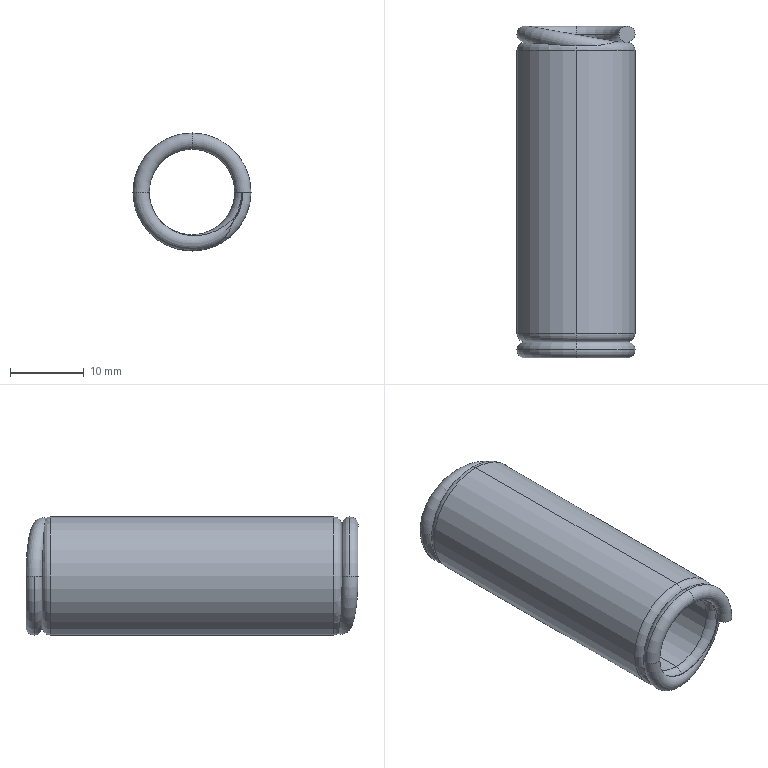Part | SolidWorks | features Revolution 5, RevCut 1 | 1 solid | 30 faces | box 16 x 45 x 16 mm | volume 4068 mm3 | torus 22 | cylinder 4 | plane 4 | commonest cylinder face diameters 11.6 x2 16 x2
STEP:
#1=CARTESIAN_POINT('',(0.,-21.4,8.));
#2=VERTEX_POINT('',#1);
#3=CARTESIAN_POINT('',(0.,-21.4,5.8));
#4=VERTEX_POINT('',#3);
#5=CARTESIAN_POINT('',(0.,-21.4,6.9));
#6=DIRECTION('',(1.,0.,0.));
#7=DIRECTION('',(0.,0.,-1.));
#8=AXIS2_PLACEMENT_3D('',#5,#6,#7);
#9=CIRCLE('',#8,1.1);
#10=EDGE_CURVE('',#2,#4,#9,.T.);
#11=ORIENTED_EDGE('',*,*,#10,.F.);
#12=CARTESIAN_POINT('',(-8.,-21.4,0.));
#13=VERTEX_POINT('',#12);
#14=CARTESIAN_POINT('',(0.,-21.4,0.));
#15=DIRECTION('',(0.,-1.,0.));
#16=DIRECTION('',(0.,0.,-1.));
#17=AXIS2_PLACEMENT_3D('',#14,#15,#16);
#18=CIRCLE('',#17,8.);
#19=EDGE_CURVE('',#2,#13,#18,.T.);
#20=ORIENTED_EDGE('',*,*,#19,.T.);
#21=CARTESIAN_POINT('',(-5.8,-21.4,0.));
#22=VERTEX_POINT('',#21);
#23=CARTESIAN_POINT('',(-6.9,-21.4,0.));
#24=DIRECTION('',(0.,0.,1.));
#25=DIRECTION('',(1.,0.,0.));
#26=AXIS2_PLACEMENT_3D('',#23,#24,#25);
#27=CIRCLE('',#26,1.1);
#28=EDGE_CURVE('',#13,#22,#27,.T.);
#29=ORIENTED_EDGE('',*,*,#28,.T.);
#30=CARTESIAN_POINT('',(0.,-21.4,0.));
#31=DIRECTION('',(0.,-1.,0.));
#32=DIRECTION('',(0.,0.,-1.));
#33=AXIS2_PLACEMENT_3D('',#30,#31,#32);
#34=CIRCLE('',#33,5.8);
#35=EDGE_CURVE('',#4,#22,#34,.T.);
#36=ORIENTED_EDGE('',*,*,#35,.F.);
#37=EDGE_LOOP('',(#11,#20,#29,#36));
#38=FACE_OUTER_BOUND('',#37,.T.);
#39=CARTESIAN_POINT('',(0.,-21.4,0.));
#40=DIRECTION('',(0.,-1.,0.));
#41=DIRECTION('',(0.,0.,-1.));
#42=AXIS2_PLACEMENT_3D('',#39,#40,#41);
#43=TOROIDAL_SURFACE('',#42,6.9,1.1);
#44=ADVANCED_FACE('',(#38),#43,.T.);
#45=CARTESIAN_POINT('',(0.,-20.3,6.9));
#46=VERTEX_POINT('',#45);
#47=CARTESIAN_POINT('',(0.,-21.4,6.9));
#48=DIRECTION('',(1.,0.,0.));
#49=DIRECTION('',(0.,0.,-1.));
#50=AXIS2_PLACEMENT_3D('',#47,#48,#49);
#51=CIRCLE('',#50,1.1);
#52=EDGE_CURVE('',#4,#46,#51,.T.);
#53=ORIENTED_EDGE('',*,*,#52,.F.);
#54=ORIENTED_EDGE('',*,*,#35,.T.);
#55=CARTESIAN_POINT('',(0.,-20.877,-5.932));
#56=VERTEX_POINT('',#55);
#57=CARTESIAN_POINT('',(0.,-20.877,-5.932));
#58=CARTESIAN_POINT('',(-0.3787,-20.912,-5.913));
#59=CARTESIAN_POINT('',(-0.7536,-20.947,-5.861));
#60=CARTESIAN_POINT('',(-1.31,-20.997,-5.731));
#61=CARTESIAN_POINT('',(-1.496,-21.014,-5.679));
#62=CARTESIAN_POINT('',(-1.858,-21.047,-5.559));
#63=CARTESIAN_POINT('',(-2.035,-21.063,-5.491));
#64=CARTESIAN_POINT('',(-2.556,-21.111,-5.263));
#65=CARTESIAN_POINT('',(-2.888,-21.141,-5.08));
#66=CARTESIAN_POINT('',(-3.522,-21.198,-4.647));
#67=CARTESIAN_POINT('',(-3.815,-21.224,-4.403));
#68=CARTESIAN_POINT('',(-4.217,-21.26,-4.));
#69=CARTESIAN_POINT('',(-4.344,-21.271,-3.859));
#70=CARTESIAN_POINT('',(-4.587,-21.293,-3.563));
#71=CARTESIAN_POINT('',(-4.702,-21.303,-3.408));
#72=CARTESIAN_POINT('',(-5.021,-21.331,-2.932));
#73=CARTESIAN_POINT('',(-5.201,-21.347,-2.598));
#74=CARTESIAN_POINT('',(-5.495,-21.373,-1.895));
#75=CARTESIAN_POINT('',(-5.609,-21.383,-1.525));
#76=CARTESIAN_POINT('',(-5.762,-21.397,-0.77));
#77=CARTESIAN_POINT('',(-5.8,-21.4,-0.3815));
#78=CARTESIAN_POINT('',(-5.8,-21.4,0.));
#79=B_SPLINE_CURVE_WITH_KNOTS('',3,(#57,#58,#59,#60,#61,#62,#63,#64,#65,#66,#67,#68,#69,#70,#71,#72,#73,#74,#75,#76,#77,#78),.UNSPECIFIED.,.F.,.F.,(4,2,2,2,2,2,2,2,2,2,4),(0.01087,0.01202,0.01259,0.01316,0.01431,0.01545,0.01602,0.01659,0.01774,0.01888,0.02003),.UNSPECIFIED.);
#80=EDGE_CURVE('',#56,#22,#79,.T.);
#81=ORIENTED_EDGE('',*,*,#80,.F.);
#82=CARTESIAN_POINT('',(0.,-20.3,-6.9));
#83=VERTEX_POINT('',#82);
#84=CARTESIAN_POINT('',(0.,-21.4,-6.9));
#85=DIRECTION('',(-1.,0.,0.));
#86=DIRECTION('',(0.,0.,1.));
#87=AXIS2_PLACEMENT_3D('',#84,#85,#86);
#88=CIRCLE('',#87,1.1);
#89=EDGE_CURVE('',#56,#83,#88,.T.);
#90=ORIENTED_EDGE('',*,*,#89,.T.);
#91=CARTESIAN_POINT('',(0.,-20.3,0.));
#92=DIRECTION('',(0.,1.,0.));
#93=DIRECTION('',(0.,0.,1.));
#94=AXIS2_PLACEMENT_3D('',#91,#92,#93);
#95=CIRCLE('',#94,6.9);
#96=EDGE_CURVE('',#83,#46,#95,.T.);
#97=ORIENTED_EDGE('',*,*,#96,.T.);
#98=EDGE_LOOP('',(#53,#54,#81,#90,#97));
#99=FACE_OUTER_BOUND('',#98,.T.);
#100=CARTESIAN_POINT('',(0.,-21.4,0.));
#101=DIRECTION('',(0.,-1.,0.));
#102=DIRECTION('',(0.,0.,-1.));
#103=AXIS2_PLACEMENT_3D('',#100,#101,#102);
#104=TOROIDAL_SURFACE('',#103,6.9,1.1);
#105=ADVANCED_FACE('',(#99),#104,.T.);
#106=CARTESIAN_POINT('',(0.,21.4,-8.));
#107=VERTEX_POINT('',#106);
#108=CARTESIAN_POINT('',(0.,21.4,-5.8));
#109=VERTEX_POINT('',#108);
#110=CARTESIAN_POINT('',(0.,21.4,-6.9));
#111=DIRECTION('',(1.,0.,0.));
#112=DIRECTION('',(0.,0.,-1.));
#113=AXIS2_PLACEMENT_3D('',#110,#111,#112);
#114=CIRCLE('',#113,1.1);
#115=EDGE_CURVE('',#107,#109,#114,.T.);
#116=ORIENTED_EDGE('',*,*,#115,.F.);
#117=CARTESIAN_POINT('',(-8.,21.4,0.));
#118=VERTEX_POINT('',#117);
#119=CARTESIAN_POINT('',(0.,21.4,0.));
#120=DIRECTION('',(0.,1.,0.));
#121=DIRECTION('',(0.,0.,1.));
#122=AXIS2_PLACEMENT_3D('',#119,#120,#121);
#123=CIRCLE('',#122,8.);
#124=EDGE_CURVE('',#107,#118,#123,.T.);
#125=ORIENTED_EDGE('',*,*,#124,.T.);
#126=CARTESIAN_POINT('',(-5.8,21.4,0.));
#127=VERTEX_POINT('',#126);
#128=CARTESIAN_POINT('',(-6.9,21.4,0.));
#129=DIRECTION('',(0.,0.,1.));
#130=DIRECTION('',(1.,0.,0.));
#131=AXIS2_PLACEMENT_3D('',#128,#129,#130);
#132=CIRCLE('',#131,1.1);
#133=EDGE_CURVE('',#127,#118,#132,.T.);
#134=ORIENTED_EDGE('',*,*,#133,.F.);
#135=CARTESIAN_POINT('',(0.,21.4,0.));
#136=DIRECTION('',(0.,1.,0.));
#137=DIRECTION('',(0.,0.,1.));
#138=AXIS2_PLACEMENT_3D('',#135,#136,#137);
#139=CIRCLE('',#138,5.8);
#140=EDGE_CURVE('',#109,#127,#139,.T.);
#141=ORIENTED_EDGE('',*,*,#140,.F.);
#142=EDGE_LOOP('',(#116,#125,#134,#141));
#143=FACE_OUTER_BOUND('',#142,.T.);
#144=CARTESIAN_POINT('',(0.,21.4,0.));
#145=DIRECTION('',(0.,1.,0.));
#146=DIRECTION('',(0.,0.,1.));
#147=AXIS2_PLACEMENT_3D('',#144,#145,#146);
#148=TOROIDAL_SURFACE('',#147,6.9,1.1);
#149=ADVANCED_FACE('',(#143),#148,.T.);
#150=CARTESIAN_POINT('',(0.,20.3,-6.9));
#151=VERTEX_POINT('',#150);
#152=CARTESIAN_POINT('',(0.,21.4,-6.9));
#153=DIRECTION('',(1.,0.,0.));
#154=DIRECTION('',(0.,0.,-1.));
#155=AXIS2_PLACEMENT_3D('',#152,#153,#154);
#156=CIRCLE('',#155,1.1);
#157=EDGE_CURVE('',#109,#151,#156,.T.);
#158=ORIENTED_EDGE('',*,*,#157,.F.);
#159=ORIENTED_EDGE('',*,*,#140,.T.);
#160=CARTESIAN_POINT('',(0.,20.877,5.932));
#161=VERTEX_POINT('',#160);
#162=CARTESIAN_POINT('',(-5.8,21.4,0.));
#163=CARTESIAN_POINT('',(-5.8,21.4,0.3854));
#164=CARTESIAN_POINT('',(-5.761,21.397,0.7711));
#165=CARTESIAN_POINT('',(-5.609,21.383,1.526));
#166=CARTESIAN_POINT('',(-5.495,21.373,1.896));
#167=CARTESIAN_POINT('',(-5.201,21.347,2.598));
#168=CARTESIAN_POINT('',(-5.021,21.331,2.933));
#169=CARTESIAN_POINT('',(-4.702,21.303,3.409));
#170=CARTESIAN_POINT('',(-4.586,21.293,3.564));
#171=CARTESIAN_POINT('',(-4.344,21.271,3.859));
#172=CARTESIAN_POINT('',(-4.216,21.26,4.));
#173=CARTESIAN_POINT('',(-3.815,21.224,4.404));
#174=CARTESIAN_POINT('',(-3.522,21.198,4.647));
#175=CARTESIAN_POINT('',(-2.888,21.141,5.08));
#176=CARTESIAN_POINT('',(-2.555,21.111,5.263));
#177=CARTESIAN_POINT('',(-2.035,21.063,5.491));
#178=CARTESIAN_POINT('',(-1.857,21.047,5.559));
#179=CARTESIAN_POINT('',(-1.496,21.014,5.679));
#180=CARTESIAN_POINT('',(-1.31,20.997,5.731));
#181=CARTESIAN_POINT('',(-0.7535,20.947,5.861));
#182=CARTESIAN_POINT('',(-0.3786,20.912,5.913));
#183=CARTESIAN_POINT('',(0.,20.877,5.932));
#184=B_SPLINE_CURVE_WITH_KNOTS('',3,(#162,#163,#164,#165,#166,#167,#168,#169,#170,#171,#172,#173,#174,#175,#176,#177,#178,#179,#180,#181,#182,#183),.UNSPECIFIED.,.F.,.F.,(4,2,2,2,2,2,2,2,2,2,4),(-0.0001166,0.001039,0.002196,0.003352,0.00393,0.004508,0.005664,0.00682,0.007398,0.007976,0.009132),.UNSPECIFIED.);
#185=EDGE_CURVE('',#127,#161,#184,.T.);
#186=ORIENTED_EDGE('',*,*,#185,.T.);
#187=CARTESIAN_POINT('',(0.,20.3,6.9));
#188=VERTEX_POINT('',#187);
#189=CARTESIAN_POINT('',(0.,21.4,6.9));
#190=DIRECTION('',(-1.,0.,0.));
#191=DIRECTION('',(0.,0.,1.));
#192=AXIS2_PLACEMENT_3D('',#189,#190,#191);
#193=CIRCLE('',#192,1.1);
#194=EDGE_CURVE('',#161,#188,#193,.T.);
#195=ORIENTED_EDGE('',*,*,#194,.T.);
#196=CARTESIAN_POINT('',(0.,20.3,0.));
#197=DIRECTION('',(0.,1.,0.));
#198=DIRECTION('',(0.,0.,1.));
#199=AXIS2_PLACEMENT_3D('',#196,#197,#198);
#200=CIRCLE('',#199,6.9);
#201=EDGE_CURVE('',#151,#188,#200,.T.);
#202=ORIENTED_EDGE('',*,*,#201,.F.);
#203=EDGE_LOOP('',(#158,#159,#186,#195,#202));
#204=FACE_OUTER_BOUND('',#203,.T.);
#205=CARTESIAN_POINT('',(0.,21.4,0.));
#206=DIRECTION('',(0.,1.,0.));
#207=DIRECTION('',(0.,0.,1.));
#208=AXIS2_PLACEMENT_3D('',#205,#206,#207);
#209=TOROIDAL_SURFACE('',#208,6.9,1.1);
#210=ADVANCED_FACE('',(#204),#209,.T.);
#211=CARTESIAN_POINT('',(5.8,21.4,0.));
#212=VERTEX_POINT('',#211);
#213=CARTESIAN_POINT('',(8.,21.4,0.));
#214=VERTEX_POINT('',#213);
#215=CARTESIAN_POINT('',(6.9,21.4,0.));
#216=DIRECTION('',(0.,0.,-1.));
#217=DIRECTION('',(-1.,0.,0.));
#218=AXIS2_PLACEMENT_3D('',#215,#216,#217);
#219=CIRCLE('',#218,1.1);
#220=EDGE_CURVE('',#212,#214,#219,.T.);
#221=ORIENTED_EDGE('',*,*,#220,.T.);
#222=CARTESIAN_POINT('',(0.,21.4,0.));
#223=DIRECTION('',(0.,1.,0.));
#224=DIRECTION('',(0.,0.,1.));
#225=AXIS2_PLACEMENT_3D('',#222,#223,#224);
#226=CIRCLE('',#225,8.);
#227=EDGE_CURVE('',#214,#107,#226,.T.);
#228=ORIENTED_EDGE('',*,*,#227,.T.);
#229=ORIENTED_EDGE('',*,*,#115,.T.);
#230=CARTESIAN_POINT('',(0.,21.4,0.));
#231=DIRECTION('',(0.,1.,0.));
#232=DIRECTION('',(0.,0.,1.));
#233=AXIS2_PLACEMENT_3D('',#230,#231,#232);
#234=CIRCLE('',#233,5.8);
#235=EDGE_CURVE('',#212,#109,#234,.T.);
#236=ORIENTED_EDGE('',*,*,#235,.F.);
#237=EDGE_LOOP('',(#221,#228,#229,#236));
#238=FACE_OUTER_BOUND('',#237,.T.);
#239=CARTESIAN_POINT('',(0.,21.4,0.));
#240=DIRECTION('',(0.,1.,0.));
#241=DIRECTION('',(0.,0.,1.));
#242=AXIS2_PLACEMENT_3D('',#239,#240,#241);
#243=TOROIDAL_SURFACE('',#242,6.9,1.1);
#244=ADVANCED_FACE('',(#238),#243,.T.);
#245=CARTESIAN_POINT('',(6.752,20.31,0.));
#246=VERTEX_POINT('',#245);
#247=CARTESIAN_POINT('',(6.9,21.4,0.));
#248=DIRECTION('',(0.,0.,-1.));
#249=DIRECTION('',(-1.,0.,0.));
#250=AXIS2_PLACEMENT_3D('',#247,#248,#249);
#251=CIRCLE('',#250,1.1);
#252=EDGE_CURVE('',#246,#212,#251,.T.);
#253=ORIENTED_EDGE('',*,*,#252,.T.);
#254=ORIENTED_EDGE('',*,*,#235,.T.);
#255=ORIENTED_EDGE('',*,*,#157,.T.);
#256=CARTESIAN_POINT('',(0.,20.3,0.));
#257=DIRECTION('',(0.,1.,0.));
#258=DIRECTION('',(0.,0.,1.));
#259=AXIS2_PLACEMENT_3D('',#256,#257,#258);
#260=CIRCLE('',#259,6.9);
#261=EDGE_CURVE('',#188,#151,#260,.T.);
#262=ORIENTED_EDGE('',*,*,#261,.F.);
#263=ORIENTED_EDGE('',*,*,#194,.F.);
#264=CARTESIAN_POINT('',(5.611,20.31,3.755));
#265=VERTEX_POINT('',#264);
#266=CARTESIAN_POINT('',(0.,20.877,5.932));
#267=CARTESIAN_POINT('',(0.2569,20.853,5.945));
#268=CARTESIAN_POINT('',(0.5168,20.829,5.943));
#269=CARTESIAN_POINT('',(1.034,20.781,5.906));
#270=CARTESIAN_POINT('',(1.289,20.757,5.873));
#271=CARTESIAN_POINT('',(1.794,20.709,5.777));
#272=CARTESIAN_POINT('',(2.043,20.685,5.714));
#273=CARTESIAN_POINT('',(2.535,20.638,5.561));
#274=CARTESIAN_POINT('',(2.779,20.615,5.469));
#275=CARTESIAN_POINT('',(3.489,20.545,5.156));
#276=CARTESIAN_POINT('',(3.934,20.501,4.897));
#277=CARTESIAN_POINT('',(4.565,20.436,4.448));
#278=CARTESIAN_POINT('',(4.769,20.415,4.287));
#279=CARTESIAN_POINT('',(5.072,20.381,4.042));
#280=CARTESIAN_POINT('',(5.172,20.37,3.959));
#281=CARTESIAN_POINT('',(5.326,20.351,3.842));
#282=CARTESIAN_POINT('',(5.379,20.345,3.803));
#283=CARTESIAN_POINT('',(5.463,20.334,3.754));
#284=CARTESIAN_POINT('',(5.493,20.33,3.738));
#285=CARTESIAN_POINT('',(5.54,20.323,3.725));
#286=CARTESIAN_POINT('',(5.557,20.32,3.723));
#287=CARTESIAN_POINT('',(5.589,20.315,3.73));
#288=CARTESIAN_POINT('',(5.603,20.312,3.741));
#289=CARTESIAN_POINT('',(5.611,20.31,3.755));
#290=B_SPLINE_CURVE_WITH_KNOTS('',3,(#266,#267,#268,#269,#270,#271,#272,#273,#274,#275,#276,#277,#278,#279,#280,#281,#282,#283,#284,#285,#286,#287,#288,#289),.UNSPECIFIED.,.F.,.F.,(4,2,2,2,2,2,2,2,2,2,2,4),(0.009132,0.009916,0.0107,0.01149,0.01227,0.01384,0.01462,0.01501,0.01521,0.01531,0.01536,0.01541),.UNSPECIFIED.);
#291=EDGE_CURVE('',#161,#265,#290,.T.);
#292=ORIENTED_EDGE('',*,*,#291,.T.);
#293=CARTESIAN_POINT('',(0.,20.31,0.));
#294=DIRECTION('',(0.,1.,0.));
#295=DIRECTION('',(0.,0.,1.));
#296=AXIS2_PLACEMENT_3D('',#293,#294,#295);
#297=CIRCLE('',#296,6.752);
#298=EDGE_CURVE('',#265,#246,#297,.T.);
#299=ORIENTED_EDGE('',*,*,#298,.T.);
#300=EDGE_LOOP('',(#253,#254,#255,#262,#263,#292,#299));
#301=FACE_OUTER_BOUND('',#300,.T.);
#302=CARTESIAN_POINT('',(0.,21.4,0.));
#303=DIRECTION('',(0.,1.,0.));
#304=DIRECTION('',(0.,0.,1.));
#305=AXIS2_PLACEMENT_3D('',#302,#303,#304);
#306=TOROIDAL_SURFACE('',#305,6.9,1.1);
#307=ADVANCED_FACE('',(#301),#306,.T.);
#308=CARTESIAN_POINT('',(8.,-21.4,0.));
#309=VERTEX_POINT('',#308);
#310=CARTESIAN_POINT('',(5.8,-21.4,0.));
#311=VERTEX_POINT('',#310);
#312=CARTESIAN_POINT('',(6.9,-21.4,0.));
#313=DIRECTION('',(0.,0.,-1.));
#314=DIRECTION('',(-1.,0.,0.));
#315=AXIS2_PLACEMENT_3D('',#312,#313,#314);
#316=CIRCLE('',#315,1.1);
#317=EDGE_CURVE('',#309,#311,#316,.T.);
#318=ORIENTED_EDGE('',*,*,#317,.F.);
#319=CARTESIAN_POINT('',(0.,-21.4,0.));
#320=DIRECTION('',(0.,-1.,0.));
#321=DIRECTION('',(0.,0.,-1.));
#322=AXIS2_PLACEMENT_3D('',#319,#320,#321);
#323=CIRCLE('',#322,8.);
#324=EDGE_CURVE('',#309,#2,#323,.T.);
#325=ORIENTED_EDGE('',*,*,#324,.T.);
#326=ORIENTED_EDGE('',*,*,#10,.T.);
#327=CARTESIAN_POINT('',(0.,-21.4,0.));
#328=DIRECTION('',(0.,-1.,0.));
#329=DIRECTION('',(0.,0.,-1.));
#330=AXIS2_PLACEMENT_3D('',#327,#328,#329);
#331=CIRCLE('',#330,5.8);
#332=EDGE_CURVE('',#311,#4,#331,.T.);
#333=ORIENTED_EDGE('',*,*,#332,.F.);
#334=EDGE_LOOP('',(#318,#325,#326,#333));
#335=FACE_OUTER_BOUND('',#334,.T.);
#336=CARTESIAN_POINT('',(0.,-21.4,0.));
#337=DIRECTION('',(0.,-1.,0.));
#338=DIRECTION('',(0.,0.,-1.));
#339=AXIS2_PLACEMENT_3D('',#336,#337,#338);
#340=TOROIDAL_SURFACE('',#339,6.9,1.1);
#341=ADVANCED_FACE('',(#335),#340,.T.);
#342=CARTESIAN_POINT('',(6.752,-20.31,0.));
#343=VERTEX_POINT('',#342);
#344=CARTESIAN_POINT('',(6.9,-21.4,0.));
#345=DIRECTION('',(0.,0.,-1.));
#346=DIRECTION('',(-1.,0.,0.));
#347=AXIS2_PLACEMENT_3D('',#344,#345,#346);
#348=CIRCLE('',#347,1.1);
#349=EDGE_CURVE('',#311,#343,#348,.T.);
#350=ORIENTED_EDGE('',*,*,#349,.F.);
#351=ORIENTED_EDGE('',*,*,#332,.T.);
#352=ORIENTED_EDGE('',*,*,#52,.T.);
#353=CARTESIAN_POINT('',(0.,-20.3,0.));
#354=DIRECTION('',(0.,1.,0.));
#355=DIRECTION('',(0.,0.,1.));
#356=AXIS2_PLACEMENT_3D('',#353,#354,#355);
#357=CIRCLE('',#356,6.9);
#358=EDGE_CURVE('',#46,#83,#357,.T.);
#359=ORIENTED_EDGE('',*,*,#358,.T.);
#360=ORIENTED_EDGE('',*,*,#89,.F.);
#361=CARTESIAN_POINT('',(5.611,-20.31,-3.755));
#362=VERTEX_POINT('',#361);
#363=CARTESIAN_POINT('',(5.611,-20.31,-3.755));
#364=CARTESIAN_POINT('',(5.603,-20.312,-3.741));
#365=CARTESIAN_POINT('',(5.589,-20.315,-3.73));
#366=CARTESIAN_POINT('',(5.557,-20.32,-3.723));
#367=CARTESIAN_POINT('',(5.54,-20.323,-3.725));
#368=CARTESIAN_POINT('',(5.493,-20.33,-3.738));
#369=CARTESIAN_POINT('',(5.463,-20.334,-3.754));
#370=CARTESIAN_POINT('',(5.379,-20.345,-3.803));
#371=CARTESIAN_POINT('',(5.326,-20.351,-3.842));
#372=CARTESIAN_POINT('',(5.172,-20.37,-3.959));
#373=CARTESIAN_POINT('',(5.072,-20.381,-4.042));
#374=CARTESIAN_POINT('',(4.769,-20.415,-4.287));
#375=CARTESIAN_POINT('',(4.565,-20.436,-4.448));
#376=CARTESIAN_POINT('',(3.934,-20.501,-4.897));
#377=CARTESIAN_POINT('',(3.489,-20.545,-5.156));
#378=CARTESIAN_POINT('',(2.779,-20.615,-5.469));
#379=CARTESIAN_POINT('',(2.535,-20.638,-5.561));
#380=CARTESIAN_POINT('',(2.043,-20.685,-5.714));
#381=CARTESIAN_POINT('',(1.794,-20.709,-5.777));
#382=CARTESIAN_POINT('',(1.289,-20.757,-5.873));
#383=CARTESIAN_POINT('',(1.034,-20.781,-5.906));
#384=CARTESIAN_POINT('',(0.5168,-20.829,-5.943));
#385=CARTESIAN_POINT('',(0.2569,-20.853,-5.945));
#386=CARTESIAN_POINT('',(0.,-20.877,-5.932));
#387=B_SPLINE_CURVE_WITH_KNOTS('',3,(#363,#364,#365,#366,#367,#368,#369,#370,#371,#372,#373,#374,#375,#376,#377,#378,#379,#380,#381,#382,#383,#384,#385,#386),.UNSPECIFIED.,.F.,.F.,(4,2,2,2,2,2,2,2,2,2,2,4),(0.004661,0.004709,0.004758,0.004855,0.005049,0.005437,0.006214,0.007766,0.008543,0.009319,0.0101,0.01087),.UNSPECIFIED.);
#388=EDGE_CURVE('',#362,#56,#387,.T.);
#389=ORIENTED_EDGE('',*,*,#388,.F.);
#390=CARTESIAN_POINT('',(0.,-20.31,0.));
#391=DIRECTION('',(0.,-1.,0.));
#392=DIRECTION('',(0.,0.,-1.));
#393=AXIS2_PLACEMENT_3D('',#390,#391,#392);
#394=CIRCLE('',#393,6.752);
#395=EDGE_CURVE('',#362,#343,#394,.T.);
#396=ORIENTED_EDGE('',*,*,#395,.T.);
#397=EDGE_LOOP('',(#350,#351,#352,#359,#360,#389,#396));
#398=FACE_OUTER_BOUND('',#397,.T.);
#399=CARTESIAN_POINT('',(0.,-21.4,0.));
#400=DIRECTION('',(0.,-1.,0.));
#401=DIRECTION('',(0.,0.,-1.));
#402=AXIS2_PLACEMENT_3D('',#399,#400,#401);
#403=TOROIDAL_SURFACE('',#402,6.9,1.1);
#404=ADVANCED_FACE('',(#398),#403,.T.);
#405=ORIENTED_EDGE('',*,*,#261,.T.);
#406=CARTESIAN_POINT('',(0.,19.2,-5.8));
#407=VERTEX_POINT('',#406);
#408=CARTESIAN_POINT('',(0.,19.2,-6.9));
#409=DIRECTION('',(1.,0.,0.));
#410=DIRECTION('',(0.,0.,-1.));
#411=AXIS2_PLACEMENT_3D('',#408,#409,#410);
#412=CIRCLE('',#411,1.1);
#413=EDGE_CURVE('',#151,#407,#412,.T.);
#414=ORIENTED_EDGE('',*,*,#413,.T.);
#415=CARTESIAN_POINT('',(0.,19.2,5.8));
#416=VERTEX_POINT('',#415);
#417=CARTESIAN_POINT('',(0.,19.2,0.));
#418=DIRECTION('',(0.,1.,0.));
#419=DIRECTION('',(0.,0.,1.));
#420=AXIS2_PLACEMENT_3D('',#417,#418,#419);
#421=CIRCLE('',#420,5.8);
#422=EDGE_CURVE('',#416,#407,#421,.T.);
#423=ORIENTED_EDGE('',*,*,#422,.F.);
#424=CARTESIAN_POINT('',(0.,19.2,6.9));
#425=DIRECTION('',(-1.,0.,0.));
#426=DIRECTION('',(0.,0.,1.));
#427=AXIS2_PLACEMENT_3D('',#424,#425,#426);
#428=CIRCLE('',#427,1.1);
#429=EDGE_CURVE('',#188,#416,#428,.T.);
#430=ORIENTED_EDGE('',*,*,#429,.F.);
#431=EDGE_LOOP('',(#405,#414,#423,#430));
#432=FACE_OUTER_BOUND('',#431,.T.);
#433=CARTESIAN_POINT('',(0.,19.2,0.));
#434=DIRECTION('',(0.,1.,0.));
#435=DIRECTION('',(0.,0.,1.));
#436=AXIS2_PLACEMENT_3D('',#433,#434,#435);
#437=TOROIDAL_SURFACE('',#436,6.9,1.1);
#438=ADVANCED_FACE('',(#432),#437,.T.);
#439=CARTESIAN_POINT('',(0.,-19.2,-5.8));
#440=VERTEX_POINT('',#439);
#441=CARTESIAN_POINT('',(0.,-19.2,5.8));
#442=VERTEX_POINT('',#441);
#443=CARTESIAN_POINT('',(0.,-19.2,0.));
#444=DIRECTION('',(0.,1.,0.));
#445=DIRECTION('',(0.,0.,1.));
#446=AXIS2_PLACEMENT_3D('',#443,#444,#445);
#447=CIRCLE('',#446,5.8);
#448=EDGE_CURVE('',#440,#442,#447,.T.);
#449=ORIENTED_EDGE('',*,*,#448,.F.);
#450=CARTESIAN_POINT('',(0.,-22.5,-5.8));
#451=DIRECTION('',(0.,1.,0.));
#452=VECTOR('',#451,1000.);
#453=LINE('',#450,#452);
#454=EDGE_CURVE('',#440,#407,#453,.T.);
#455=ORIENTED_EDGE('',*,*,#454,.T.);
#456=CARTESIAN_POINT('',(0.,19.2,0.));
#457=DIRECTION('',(0.,1.,0.));
#458=DIRECTION('',(0.,0.,1.));
#459=AXIS2_PLACEMENT_3D('',#456,#457,#458);
#460=CIRCLE('',#459,5.8);
#461=EDGE_CURVE('',#407,#416,#460,.T.);
#462=ORIENTED_EDGE('',*,*,#461,.T.);
#463=CARTESIAN_POINT('',(0.,-22.5,5.8));
#464=DIRECTION('',(0.,1.,0.));
#465=VECTOR('',#464,1000.);
#466=LINE('',#463,#465);
#467=EDGE_CURVE('',#442,#416,#466,.T.);
#468=ORIENTED_EDGE('',*,*,#467,.F.);
#469=EDGE_LOOP('',(#449,#455,#462,#468));
#470=FACE_OUTER_BOUND('',#469,.T.);
#471=CARTESIAN_POINT('',(0.,-22.5,0.));
#472=DIRECTION('',(0.,1.,0.));
#473=DIRECTION('',(0.,0.,1.));
#474=AXIS2_PLACEMENT_3D('',#471,#472,#473);
#475=CYLINDRICAL_SURFACE('',#474,5.8);
#476=ADVANCED_FACE('',(#470),#475,.F.);
#477=CARTESIAN_POINT('',(0.,-19.2,0.));
#478=DIRECTION('',(0.,1.,0.));
#479=DIRECTION('',(0.,0.,1.));
#480=AXIS2_PLACEMENT_3D('',#477,#478,#479);
#481=CIRCLE('',#480,5.8);
#482=EDGE_CURVE('',#442,#440,#481,.T.);
#483=ORIENTED_EDGE('',*,*,#482,.T.);
#484=CARTESIAN_POINT('',(0.,-19.2,-6.9));
#485=DIRECTION('',(1.,0.,0.));
#486=DIRECTION('',(0.,0.,-1.));
#487=AXIS2_PLACEMENT_3D('',#484,#485,#486);
#488=CIRCLE('',#487,1.1);
#489=EDGE_CURVE('',#440,#83,#488,.T.);
#490=ORIENTED_EDGE('',*,*,#489,.T.);
#491=ORIENTED_EDGE('',*,*,#358,.F.);
#492=CARTESIAN_POINT('',(0.,-19.2,6.9));
#493=DIRECTION('',(-1.,0.,0.));
#494=DIRECTION('',(0.,0.,1.));
#495=AXIS2_PLACEMENT_3D('',#492,#493,#494);
#496=CIRCLE('',#495,1.1);
#497=EDGE_CURVE('',#442,#46,#496,.T.);
#498=ORIENTED_EDGE('',*,*,#497,.F.);
#499=EDGE_LOOP('',(#483,#490,#491,#498));
#500=FACE_OUTER_BOUND('',#499,.T.);
#501=CARTESIAN_POINT('',(0.,-19.2,0.));
#502=DIRECTION('',(0.,1.,0.));
#503=DIRECTION('',(0.,0.,1.));
#504=AXIS2_PLACEMENT_3D('',#501,#502,#503);
#505=TOROIDAL_SURFACE('',#504,6.9,1.1);
#506=ADVANCED_FACE('',(#500),#505,.T.);
#507=ORIENTED_EDGE('',*,*,#324,.F.);
#508=CARTESIAN_POINT('',(7.005,-20.305,0.));
#509=VERTEX_POINT('',#508);
#510=CARTESIAN_POINT('',(6.9,-21.4,0.));
#511=DIRECTION('',(0.,0.,-1.));
#512=DIRECTION('',(-1.,0.,0.));
#513=AXIS2_PLACEMENT_3D('',#510,#511,#512);
#514=CIRCLE('',#513,1.1);
#515=EDGE_CURVE('',#509,#309,#514,.T.);
#516=ORIENTED_EDGE('',*,*,#515,.F.);
#517=CARTESIAN_POINT('',(0.,-20.305,7.005));
#518=VERTEX_POINT('',#517);
#519=CARTESIAN_POINT('',(0.,-20.305,0.));
#520=DIRECTION('',(0.,-1.,0.));
#521=DIRECTION('',(0.,0.,-1.));
#522=AXIS2_PLACEMENT_3D('',#519,#520,#521);
#523=CIRCLE('',#522,7.005);
#524=EDGE_CURVE('',#509,#518,#523,.T.);
#525=ORIENTED_EDGE('',*,*,#524,.T.);
#526=CARTESIAN_POINT('',(0.,-21.4,6.9));
#527=DIRECTION('',(1.,0.,0.));
#528=DIRECTION('',(0.,0.,-1.));
#529=AXIS2_PLACEMENT_3D('',#526,#527,#528);
#530=CIRCLE('',#529,1.1);
#531=EDGE_CURVE('',#518,#2,#530,.T.);
#532=ORIENTED_EDGE('',*,*,#531,.T.);
#533=EDGE_LOOP('',(#507,#516,#525,#532));
#534=FACE_OUTER_BOUND('',#533,.T.);
#535=CARTESIAN_POINT('',(0.,-21.4,0.));
#536=DIRECTION('',(0.,-1.,0.));
#537=DIRECTION('',(0.,0.,-1.));
#538=AXIS2_PLACEMENT_3D('',#535,#536,#537);
#539=TOROIDAL_SURFACE('',#538,6.9,1.1);
#540=ADVANCED_FACE('',(#534),#539,.T.);
#541=ORIENTED_EDGE('',*,*,#227,.F.);
#542=CARTESIAN_POINT('',(7.005,20.305,0.));
#543=VERTEX_POINT('',#542);
#544=CARTESIAN_POINT('',(6.9,21.4,0.));
#545=DIRECTION('',(0.,0.,-1.));
#546=DIRECTION('',(-1.,0.,0.));
#547=AXIS2_PLACEMENT_3D('',#544,#545,#546);
#548=CIRCLE('',#547,1.1);
#549=EDGE_CURVE('',#214,#543,#548,.T.);
#550=ORIENTED_EDGE('',*,*,#549,.T.);
#551=CARTESIAN_POINT('',(0.,20.305,-7.005));
#552=VERTEX_POINT('',#551);
#553=CARTESIAN_POINT('',(0.,20.305,0.));
#554=DIRECTION('',(0.,-1.,0.));
#555=DIRECTION('',(0.,0.,1.));
#556=AXIS2_PLACEMENT_3D('',#553,#554,#555);
#557=CIRCLE('',#556,7.005);
#558=EDGE_CURVE('',#552,#543,#557,.T.);
#559=ORIENTED_EDGE('',*,*,#558,.F.);
#560=CARTESIAN_POINT('',(0.,21.4,-6.9));
#561=DIRECTION('',(1.,0.,0.));
#562=DIRECTION('',(0.,0.,-1.));
#563=AXIS2_PLACEMENT_3D('',#560,#561,#562);
#564=CIRCLE('',#563,1.1);
#565=EDGE_CURVE('',#552,#107,#564,.T.);
#566=ORIENTED_EDGE('',*,*,#565,.T.);
#567=EDGE_LOOP('',(#541,#550,#559,#566));
#568=FACE_OUTER_BOUND('',#567,.T.);
#569=CARTESIAN_POINT('',(0.,21.4,0.));
#570=DIRECTION('',(0.,1.,0.));
#571=DIRECTION('',(0.,0.,1.));
#572=AXIS2_PLACEMENT_3D('',#569,#570,#571);
#573=TOROIDAL_SURFACE('',#572,6.9,1.1);
#574=ADVANCED_FACE('',(#568),#573,.T.);
#575=CARTESIAN_POINT('',(5.522,-20.31,-4.138));
#576=VERTEX_POINT('',#575);
#577=CARTESIAN_POINT('',(0.,-19.805,-7.825));
#578=VERTEX_POINT('',#577);
#579=CARTESIAN_POINT('',(5.522,-20.31,-4.138));
#580=CARTESIAN_POINT('',(5.427,-20.31,-4.423));
#581=CARTESIAN_POINT('',(5.321,-20.296,-4.708));
#582=CARTESIAN_POINT('',(5.069,-20.242,-5.25));
#583=CARTESIAN_POINT('',(4.923,-20.203,-5.508));
#584=CARTESIAN_POINT('',(4.663,-20.135,-5.872));
#585=CARTESIAN_POINT('',(4.569,-20.112,-5.989));
#586=CARTESIAN_POINT('',(4.37,-20.065,-6.211));
#587=CARTESIAN_POINT('',(4.266,-20.042,-6.316));
#588=CARTESIAN_POINT('',(3.937,-19.977,-6.614));
#589=CARTESIAN_POINT('',(3.698,-19.938,-6.79));
#590=CARTESIAN_POINT('',(2.926,-19.841,-7.26));
#591=CARTESIAN_POINT('',(2.371,-19.808,-7.48));
#592=CARTESIAN_POINT('',(1.493,-19.788,-7.698));
#593=CARTESIAN_POINT('',(1.195,-19.787,-7.751));
#594=CARTESIAN_POINT('',(0.6001,-19.791,-7.817));
#595=CARTESIAN_POINT('',(0.3009,-19.797,-7.831));
#596=CARTESIAN_POINT('',(0.,-19.805,-7.825));
#597=B_SPLINE_CURVE_WITH_KNOTS('',3,(#579,#580,#581,#582,#583,#584,#585,#586,#587,#588,#589,#590,#591,#592,#593,#594,#595,#596),.UNSPECIFIED.,.F.,.F.,(4,2,2,2,2,2,2,2,4),(0.004219,0.005119,0.006018,0.006468,0.006918,0.007817,0.009616,0.01052,0.01142),.UNSPECIFIED.);
#598=EDGE_CURVE('',#576,#578,#597,.T.);
#599=ORIENTED_EDGE('',*,*,#598,.T.);
#600=CARTESIAN_POINT('',(0.,-19.21,-8.));
#601=VERTEX_POINT('',#600);
#602=CARTESIAN_POINT('',(0.,-19.21,-6.9));
#603=DIRECTION('',(1.,0.,0.));
#604=DIRECTION('',(0.,0.,-1.));
#605=AXIS2_PLACEMENT_3D('',#602,#603,#604);
#606=CIRCLE('',#605,1.1);
#607=EDGE_CURVE('',#578,#601,#606,.T.);
#608=ORIENTED_EDGE('',*,*,#607,.T.);
#609=CARTESIAN_POINT('',(0.,-19.21,8.));
#610=VERTEX_POINT('',#609);
#611=CARTESIAN_POINT('',(0.,-19.21,0.));
#612=DIRECTION('',(0.,1.,0.));
#613=DIRECTION('',(0.,0.,1.));
#614=AXIS2_PLACEMENT_3D('',#611,#612,#613);
#615=CIRCLE('',#614,8.);
#616=EDGE_CURVE('',#610,#601,#615,.T.);
#617=ORIENTED_EDGE('',*,*,#616,.F.);
#618=CARTESIAN_POINT('',(0.,-19.21,6.9));
#619=DIRECTION('',(-1.,0.,0.));
#620=DIRECTION('',(0.,0.,1.));
#621=AXIS2_PLACEMENT_3D('',#618,#619,#620);
#622=CIRCLE('',#621,1.1);
#623=EDGE_CURVE('',#518,#610,#622,.T.);
#624=ORIENTED_EDGE('',*,*,#623,.F.);
#625=ORIENTED_EDGE('',*,*,#524,.F.);
#626=CARTESIAN_POINT('',(6.9,-20.31,0.));
#627=VERTEX_POINT('',#626);
#628=CARTESIAN_POINT('',(6.9,-19.21,0.));
#629=DIRECTION('',(0.,0.,-1.));
#630=DIRECTION('',(-1.,0.,0.));
#631=AXIS2_PLACEMENT_3D('',#628,#629,#630);
#632=CIRCLE('',#631,1.1);
#633=EDGE_CURVE('',#509,#627,#632,.T.);
#634=ORIENTED_EDGE('',*,*,#633,.T.);
#635=CARTESIAN_POINT('',(0.,-20.31,0.));
#636=DIRECTION('',(0.,1.,0.));
#637=DIRECTION('',(0.,0.,1.));
#638=AXIS2_PLACEMENT_3D('',#635,#636,#637);
#639=CIRCLE('',#638,6.9);
#640=EDGE_CURVE('',#627,#576,#639,.T.);
#641=ORIENTED_EDGE('',*,*,#640,.T.);
#642=EDGE_LOOP('',(#599,#608,#617,#624,#625,#634,#641));
#643=FACE_OUTER_BOUND('',#642,.T.);
#644=CARTESIAN_POINT('',(0.,-19.21,0.));
#645=DIRECTION('',(0.,1.,0.));
#646=DIRECTION('',(0.,0.,1.));
#647=AXIS2_PLACEMENT_3D('',#644,#645,#646);
#648=TOROIDAL_SURFACE('',#647,6.9,1.1);
#649=ADVANCED_FACE('',(#643),#648,.T.);
#650=ORIENTED_EDGE('',*,*,#616,.T.);
#651=CARTESIAN_POINT('',(0.,19.21,-8.));
#652=VERTEX_POINT('',#651);
#653=CARTESIAN_POINT('',(0.,-20.31,-8.));
#654=DIRECTION('',(0.,1.,0.));
#655=VECTOR('',#654,1000.);
#656=LINE('',#653,#655);
#657=EDGE_CURVE('',#601,#652,#656,.T.);
#658=ORIENTED_EDGE('',*,*,#657,.T.);
#659=CARTESIAN_POINT('',(0.,19.21,8.));
#660=VERTEX_POINT('',#659);
#661=CARTESIAN_POINT('',(0.,19.21,0.));
#662=DIRECTION('',(0.,1.,0.));
#663=DIRECTION('',(0.,0.,1.));
#664=AXIS2_PLACEMENT_3D('',#661,#662,#663);
#665=CIRCLE('',#664,8.);
#666=EDGE_CURVE('',#660,#652,#665,.T.);
#667=ORIENTED_EDGE('',*,*,#666,.F.);
#668=CARTESIAN_POINT('',(0.,-20.31,8.));
#669=DIRECTION('',(0.,1.,0.));
#670=VECTOR('',#669,1000.);
#671=LINE('',#668,#670);
#672=EDGE_CURVE('',#610,#660,#671,.T.);
#673=ORIENTED_EDGE('',*,*,#672,.F.);
#674=EDGE_LOOP('',(#650,#658,#667,#673));
#675=FACE_OUTER_BOUND('',#674,.T.);
#676=CARTESIAN_POINT('',(0.,-20.31,0.));
#677=DIRECTION('',(0.,1.,0.));
#678=DIRECTION('',(0.,0.,1.));
#679=AXIS2_PLACEMENT_3D('',#676,#677,#678);
#680=CYLINDRICAL_SURFACE('',#679,8.);
#681=ADVANCED_FACE('',(#675),#680,.T.);
#682=ORIENTED_EDGE('',*,*,#666,.T.);
#683=CARTESIAN_POINT('',(0.,19.21,-6.9));
#684=DIRECTION('',(1.,0.,0.));
#685=DIRECTION('',(0.,0.,-1.));
#686=AXIS2_PLACEMENT_3D('',#683,#684,#685);
#687=CIRCLE('',#686,1.1);
#688=EDGE_CURVE('',#652,#552,#687,.T.);
#689=ORIENTED_EDGE('',*,*,#688,.T.);
#690=ORIENTED_EDGE('',*,*,#558,.T.);
#691=CARTESIAN_POINT('',(6.9,20.31,0.));
#692=VERTEX_POINT('',#691);
#693=CARTESIAN_POINT('',(6.9,19.21,0.));
#694=DIRECTION('',(0.,0.,-1.));
#695=DIRECTION('',(-1.,0.,0.));
#696=AXIS2_PLACEMENT_3D('',#693,#694,#695);
#697=CIRCLE('',#696,1.1);
#698=EDGE_CURVE('',#692,#543,#697,.T.);
#699=ORIENTED_EDGE('',*,*,#698,.F.);
#700=CARTESIAN_POINT('',(5.522,20.31,4.138));
#701=VERTEX_POINT('',#700);
#702=CARTESIAN_POINT('',(0.,20.31,0.));
#703=DIRECTION('',(0.,1.,0.));
#704=DIRECTION('',(0.,0.,1.));
#705=AXIS2_PLACEMENT_3D('',#702,#703,#704);
#706=CIRCLE('',#705,6.9);
#707=EDGE_CURVE('',#701,#692,#706,.T.);
#708=ORIENTED_EDGE('',*,*,#707,.F.);
#709=CARTESIAN_POINT('',(0.,19.805,7.825));
#710=VERTEX_POINT('',#709);
#711=CARTESIAN_POINT('',(0.,19.805,7.825));
#712=CARTESIAN_POINT('',(0.6036,19.788,7.836));
#713=CARTESIAN_POINT('',(1.197,19.782,7.771));
#714=CARTESIAN_POINT('',(2.07,19.801,7.555));
#715=CARTESIAN_POINT('',(2.36,19.813,7.462));
#716=CARTESIAN_POINT('',(2.917,19.849,7.236));
#717=CARTESIAN_POINT('',(3.184,19.874,7.103));
#718=CARTESIAN_POINT('',(3.695,19.937,6.792));
#719=CARTESIAN_POINT('',(3.94,19.977,6.611));
#720=CARTESIAN_POINT('',(4.379,20.065,6.213));
#721=CARTESIAN_POINT('',(4.575,20.113,5.994));
#722=CARTESIAN_POINT('',(4.921,20.202,5.511));
#723=CARTESIAN_POINT('',(5.071,20.243,5.247));
#724=CARTESIAN_POINT('',(5.322,20.297,4.704));
#725=CARTESIAN_POINT('',(5.427,20.31,4.423));
#726=CARTESIAN_POINT('',(5.522,20.31,4.138));
#727=B_SPLINE_CURVE_WITH_KNOTS('',3,(#711,#712,#713,#714,#715,#716,#717,#718,#719,#720,#721,#722,#723,#724,#725,#726),.UNSPECIFIED.,.F.,.F.,(4,2,2,2,2,2,2,4),(0.01178,0.01358,0.01448,0.01538,0.01628,0.01718,0.01808,0.01898),.UNSPECIFIED.);
#728=EDGE_CURVE('',#710,#701,#727,.T.);
#729=ORIENTED_EDGE('',*,*,#728,.F.);
#730=CARTESIAN_POINT('',(0.,19.21,6.9));
#731=DIRECTION('',(-1.,0.,0.));
#732=DIRECTION('',(0.,0.,1.));
#733=AXIS2_PLACEMENT_3D('',#730,#731,#732);
#734=CIRCLE('',#733,1.1);
#735=EDGE_CURVE('',#660,#710,#734,.T.);
#736=ORIENTED_EDGE('',*,*,#735,.F.);
#737=EDGE_LOOP('',(#682,#689,#690,#699,#708,#729,#736));
#738=FACE_OUTER_BOUND('',#737,.T.);
#739=CARTESIAN_POINT('',(0.,19.21,0.));
#740=DIRECTION('',(0.,1.,0.));
#741=DIRECTION('',(0.,0.,1.));
#742=AXIS2_PLACEMENT_3D('',#739,#740,#741);
#743=TOROIDAL_SURFACE('',#742,6.9,1.1);
#744=ADVANCED_FACE('',(#738),#743,.T.);
#745=ORIENTED_EDGE('',*,*,#298,.F.);
#746=CARTESIAN_POINT('',(5.522,20.31,4.138));
#747=CARTESIAN_POINT('',(5.542,20.31,4.076));
#748=CARTESIAN_POINT('',(5.561,20.31,4.013));
#749=CARTESIAN_POINT('',(5.592,20.31,3.885));
#750=CARTESIAN_POINT('',(5.605,20.31,3.82));
#751=CARTESIAN_POINT('',(5.611,20.31,3.755));
#752=B_SPLINE_CURVE_WITH_KNOTS('',3,(#746,#747,#748,#749,#750,#751),.UNSPECIFIED.,.F.,.F.,(4,2,4),(0.06523,0.06543,0.06563),.UNSPECIFIED.);
#753=EDGE_CURVE('',#701,#265,#752,.T.);
#754=ORIENTED_EDGE('',*,*,#753,.F.);
#755=ORIENTED_EDGE('',*,*,#707,.T.);
#756=CARTESIAN_POINT('',(0.,20.31,0.));
#757=DIRECTION('',(1.,0.,0.));
#758=VECTOR('',#757,1000.);
#759=LINE('',#756,#758);
#760=EDGE_CURVE('',#246,#692,#759,.T.);
#761=ORIENTED_EDGE('',*,*,#760,.F.);
#762=EDGE_LOOP('',(#745,#754,#755,#761));
#763=FACE_OUTER_BOUND('',#762,.T.);
#764=CARTESIAN_POINT('',(0.,20.31,0.));
#765=DIRECTION('',(0.,-1.,0.));
#766=DIRECTION('',(0.,0.,-1.));
#767=AXIS2_PLACEMENT_3D('',#764,#765,#766);
#768=PLANE('',#767);
#769=ADVANCED_FACE('',(#763),#768,.F.);
#770=ORIENTED_EDGE('',*,*,#395,.F.);
#771=CARTESIAN_POINT('',(5.611,-20.31,-3.755));
#772=CARTESIAN_POINT('',(5.604,-20.31,-3.821));
#773=CARTESIAN_POINT('',(5.592,-20.31,-3.886));
#774=CARTESIAN_POINT('',(5.561,-20.31,-4.013));
#775=CARTESIAN_POINT('',(5.542,-20.31,-4.076));
#776=CARTESIAN_POINT('',(5.522,-20.31,-4.138));
#777=B_SPLINE_CURVE_WITH_KNOTS('',3,(#771,#772,#773,#774,#775,#776),.UNSPECIFIED.,.F.,.F.,(4,2,4),(0.006289,0.006487,0.006684),.UNSPECIFIED.);
#778=EDGE_CURVE('',#362,#576,#777,.T.);
#779=ORIENTED_EDGE('',*,*,#778,.T.);
#780=ORIENTED_EDGE('',*,*,#640,.F.);
#781=CARTESIAN_POINT('',(6.9,-20.31,0.));
#782=DIRECTION('',(-1.,0.,0.));
#783=VECTOR('',#782,1000.);
#784=LINE('',#781,#783);
#785=EDGE_CURVE('',#627,#343,#784,.T.);
#786=ORIENTED_EDGE('',*,*,#785,.T.);
#787=EDGE_LOOP('',(#770,#779,#780,#786));
#788=FACE_OUTER_BOUND('',#787,.T.);
#789=CARTESIAN_POINT('',(6.9,-20.31,0.));
#790=DIRECTION('',(0.,1.,0.));
#791=DIRECTION('',(0.,0.,1.));
#792=AXIS2_PLACEMENT_3D('',#789,#790,#791);
#793=PLANE('',#792);
#794=ADVANCED_FACE('',(#788),#793,.F.);
#795=ORIENTED_EDGE('',*,*,#185,.F.);
#796=ORIENTED_EDGE('',*,*,#133,.T.);
#797=CARTESIAN_POINT('',(-7.005,20.305,0.));
#798=VERTEX_POINT('',#797);
#799=CARTESIAN_POINT('',(-6.9,21.4,0.));
#800=DIRECTION('',(0.,0.,1.));
#801=DIRECTION('',(1.,0.,0.));
#802=AXIS2_PLACEMENT_3D('',#799,#800,#801);
#803=CIRCLE('',#802,1.1);
#804=EDGE_CURVE('',#118,#798,#803,.T.);
#805=ORIENTED_EDGE('',*,*,#804,.T.);
#806=CARTESIAN_POINT('',(-7.005,20.305,0.));
#807=CARTESIAN_POINT('',(-7.005,20.305,0.4923));
#808=CARTESIAN_POINT('',(-7.002,20.3,0.9842));
#809=CARTESIAN_POINT('',(-6.893,20.283,1.96));
#810=CARTESIAN_POINT('',(-6.79,20.269,2.447));
#811=CARTESIAN_POINT('',(-6.49,20.236,3.379));
#812=CARTESIAN_POINT('',(-6.293,20.216,3.826));
#813=CARTESIAN_POINT('',(-5.802,20.169,4.684));
#814=CARTESIAN_POINT('',(-5.516,20.144,5.081));
#815=CARTESIAN_POINT('',(-5.03,20.103,5.627));
#816=CARTESIAN_POINT('',(-4.858,20.089,5.801));
#817=CARTESIAN_POINT('',(-4.495,20.06,6.132));
#818=CARTESIAN_POINT('',(-4.304,20.045,6.289));
#819=CARTESIAN_POINT('',(-3.713,20.001,6.725));
#820=CARTESIAN_POINT('',(-3.293,19.971,6.972));
#821=CARTESIAN_POINT('',(-2.625,19.928,7.279));
#822=CARTESIAN_POINT('',(-2.394,19.914,7.37));
#823=CARTESIAN_POINT('',(-1.929,19.887,7.528));
#824=CARTESIAN_POINT('',(-1.694,19.874,7.594));
#825=CARTESIAN_POINT('',(-1.219,19.851,7.702));
#826=CARTESIAN_POINT('',(-0.9788,19.84,7.744));
#827=CARTESIAN_POINT('',(-0.4932,19.82,7.803));
#828=CARTESIAN_POINT('',(-0.2466,19.812,7.821));
#829=CARTESIAN_POINT('',(0.,19.805,7.825));
#830=B_SPLINE_CURVE_WITH_KNOTS('',3,(#806,#807,#808,#809,#810,#811,#812,#813,#814,#815,#816,#817,#818,#819,#820,#821,#822,#823,#824,#825,#826,#827,#828,#829),.UNSPECIFIED.,.F.,.F.,(4,2,2,2,2,2,2,2,2,2,2,4),(0.000000199,0.001472,0.002944,0.004416,0.005888,0.006624,0.00736,0.008832,0.009568,0.0103,0.01104,0.01178),.UNSPECIFIED.);
#831=EDGE_CURVE('',#798,#710,#830,.T.);
#832=ORIENTED_EDGE('',*,*,#831,.T.);
#833=ORIENTED_EDGE('',*,*,#728,.T.);
#834=ORIENTED_EDGE('',*,*,#753,.T.);
#835=ORIENTED_EDGE('',*,*,#291,.F.);
#836=EDGE_LOOP('',(#795,#796,#805,#832,#833,#834,#835));
#837=FACE_OUTER_BOUND('',#836,.T.);
#838=CARTESIAN_POINT('',(-0.2081,20.22,0.));
#839=DIRECTION('',(-0.1736,-0.9848,0.));
#840=DIRECTION('',(0.9848,-0.1736,0.));
#841=AXIS2_PLACEMENT_3D('',#838,#839,#840);
#842=TOROIDAL_SURFACE('',#841,6.795,1.1);
#843=ADVANCED_FACE('',(#837),#842,.T.);
#844=ORIENTED_EDGE('',*,*,#778,.F.);
#845=ORIENTED_EDGE('',*,*,#388,.T.);
#846=ORIENTED_EDGE('',*,*,#80,.T.);
#847=ORIENTED_EDGE('',*,*,#28,.F.);
#848=CARTESIAN_POINT('',(-7.005,-20.305,0.));
#849=VERTEX_POINT('',#848);
#850=CARTESIAN_POINT('',(-6.9,-21.4,0.));
#851=DIRECTION('',(0.,0.,1.));
#852=DIRECTION('',(1.,0.,0.));
#853=AXIS2_PLACEMENT_3D('',#850,#851,#852);
#854=CIRCLE('',#853,1.1);
#855=EDGE_CURVE('',#849,#13,#854,.T.);
#856=ORIENTED_EDGE('',*,*,#855,.F.);
#857=CARTESIAN_POINT('',(0.,-19.805,-7.825));
#858=CARTESIAN_POINT('',(-0.2463,-19.812,-7.821));
#859=CARTESIAN_POINT('',(-0.4936,-19.82,-7.803));
#860=CARTESIAN_POINT('',(-0.9801,-19.84,-7.744));
#861=CARTESIAN_POINT('',(-1.221,-19.851,-7.702));
#862=CARTESIAN_POINT('',(-1.696,-19.874,-7.593));
#863=CARTESIAN_POINT('',(-1.932,-19.887,-7.527));
#864=CARTESIAN_POINT('',(-2.397,-19.914,-7.369));
#865=CARTESIAN_POINT('',(-2.627,-19.928,-7.278));
#866=CARTESIAN_POINT('',(-3.295,-19.971,-6.971));
#867=CARTESIAN_POINT('',(-3.715,-20.001,-6.724));
#868=CARTESIAN_POINT('',(-4.305,-20.045,-6.288));
#869=CARTESIAN_POINT('',(-4.496,-20.06,-6.131));
#870=CARTESIAN_POINT('',(-4.859,-20.089,-5.799));
#871=CARTESIAN_POINT('',(-5.031,-20.103,-5.625));
#872=CARTESIAN_POINT('',(-5.517,-20.144,-5.079));
#873=CARTESIAN_POINT('',(-5.803,-20.169,-4.683));
#874=CARTESIAN_POINT('',(-6.294,-20.216,-3.825));
#875=CARTESIAN_POINT('',(-6.49,-20.236,-3.378));
#876=CARTESIAN_POINT('',(-6.715,-20.261,-2.681));
#877=CARTESIAN_POINT('',(-6.778,-20.268,-2.445));
#878=CARTESIAN_POINT('',(-6.88,-20.281,-1.963));
#879=CARTESIAN_POINT('',(-6.919,-20.287,-1.718));
#880=CARTESIAN_POINT('',(-7.002,-20.3,-0.985));
#881=CARTESIAN_POINT('',(-7.005,-20.305,-0.4926));
#882=CARTESIAN_POINT('',(-7.005,-20.305,0.));
#883=B_SPLINE_CURVE_WITH_KNOTS('',3,(#857,#858,#859,#860,#861,#862,#863,#864,#865,#866,#867,#868,#869,#870,#871,#872,#873,#874,#875,#876,#877,#878,#879,#880,#881,#882),.UNSPECIFIED.,.F.,.F.,(4,2,2,2,2,2,2,2,2,2,2,2,4),(0.01142,0.01215,0.01289,0.01362,0.01436,0.01583,0.01657,0.01731,0.01878,0.02025,0.02099,0.02172,0.0232),.UNSPECIFIED.);
#884=EDGE_CURVE('',#578,#849,#883,.T.);
#885=ORIENTED_EDGE('',*,*,#884,.F.);
#886=ORIENTED_EDGE('',*,*,#598,.F.);
#887=EDGE_LOOP('',(#844,#845,#846,#847,#856,#885,#886));
#888=FACE_OUTER_BOUND('',#887,.T.);
#889=CARTESIAN_POINT('',(-0.2081,-20.22,0.));
#890=DIRECTION('',(-0.1736,0.9848,0.));
#891=DIRECTION('',(-0.9848,-0.1736,0.));
#892=AXIS2_PLACEMENT_3D('',#889,#890,#891);
#893=TOROIDAL_SURFACE('',#892,6.795,1.1);
#894=ADVANCED_FACE('',(#888),#893,.T.);
#895=ORIENTED_EDGE('',*,*,#688,.F.);
#896=CARTESIAN_POINT('',(0.,19.21,0.));
#897=DIRECTION('',(0.,1.,0.));
#898=DIRECTION('',(0.,0.,1.));
#899=AXIS2_PLACEMENT_3D('',#896,#897,#898);
#900=CIRCLE('',#899,8.);
#901=EDGE_CURVE('',#652,#660,#900,.T.);
#902=ORIENTED_EDGE('',*,*,#901,.T.);
#903=ORIENTED_EDGE('',*,*,#735,.T.);
#904=ORIENTED_EDGE('',*,*,#831,.F.);
#905=CARTESIAN_POINT('',(0.,20.305,0.));
#906=DIRECTION('',(0.,-1.,0.));
#907=DIRECTION('',(0.,0.,1.));
#908=AXIS2_PLACEMENT_3D('',#905,#906,#907);
#909=CIRCLE('',#908,7.005);
#910=EDGE_CURVE('',#798,#552,#909,.T.);
#911=ORIENTED_EDGE('',*,*,#910,.T.);
#912=EDGE_LOOP('',(#895,#902,#903,#904,#911));
#913=FACE_OUTER_BOUND('',#912,.T.);
#914=CARTESIAN_POINT('',(0.,19.21,0.));
#915=DIRECTION('',(0.,1.,0.));
#916=DIRECTION('',(0.,0.,1.));
#917=AXIS2_PLACEMENT_3D('',#914,#915,#916);
#918=TOROIDAL_SURFACE('',#917,6.9,1.1);
#919=ADVANCED_FACE('',(#913),#918,.T.);
#920=ORIENTED_EDGE('',*,*,#657,.F.);
#921=CARTESIAN_POINT('',(0.,-19.21,0.));
#922=DIRECTION('',(0.,1.,0.));
#923=DIRECTION('',(0.,0.,1.));
#924=AXIS2_PLACEMENT_3D('',#921,#922,#923);
#925=CIRCLE('',#924,8.);
#926=EDGE_CURVE('',#601,#610,#925,.T.);
#927=ORIENTED_EDGE('',*,*,#926,.T.);
#928=ORIENTED_EDGE('',*,*,#672,.T.);
#929=ORIENTED_EDGE('',*,*,#901,.F.);
#930=EDGE_LOOP('',(#920,#927,#928,#929));
#931=FACE_OUTER_BOUND('',#930,.T.);
#932=CARTESIAN_POINT('',(0.,-20.31,0.));
#933=DIRECTION('',(0.,1.,0.));
#934=DIRECTION('',(0.,0.,1.));
#935=AXIS2_PLACEMENT_3D('',#932,#933,#934);
#936=CYLINDRICAL_SURFACE('',#935,8.);
#937=ADVANCED_FACE('',(#931),#936,.T.);
#938=ORIENTED_EDGE('',*,*,#607,.F.);
#939=ORIENTED_EDGE('',*,*,#884,.T.);
#940=CARTESIAN_POINT('',(0.,-20.305,0.));
#941=DIRECTION('',(0.,-1.,0.));
#942=DIRECTION('',(0.,0.,-1.));
#943=AXIS2_PLACEMENT_3D('',#940,#941,#942);
#944=CIRCLE('',#943,7.005);
#945=EDGE_CURVE('',#518,#849,#944,.T.);
#946=ORIENTED_EDGE('',*,*,#945,.F.);
#947=ORIENTED_EDGE('',*,*,#623,.T.);
#948=ORIENTED_EDGE('',*,*,#926,.F.);
#949=EDGE_LOOP('',(#938,#939,#946,#947,#948));
#950=FACE_OUTER_BOUND('',#949,.T.);
#951=CARTESIAN_POINT('',(0.,-19.21,0.));
#952=DIRECTION('',(0.,1.,0.));
#953=DIRECTION('',(0.,0.,1.));
#954=AXIS2_PLACEMENT_3D('',#951,#952,#953);
#955=TOROIDAL_SURFACE('',#954,6.9,1.1);
#956=ADVANCED_FACE('',(#950),#955,.T.);
#957=ORIENTED_EDGE('',*,*,#124,.F.);
#958=ORIENTED_EDGE('',*,*,#565,.F.);
#959=ORIENTED_EDGE('',*,*,#910,.F.);
#960=ORIENTED_EDGE('',*,*,#804,.F.);
#961=EDGE_LOOP('',(#957,#958,#959,#960));
#962=FACE_OUTER_BOUND('',#961,.T.);
#963=CARTESIAN_POINT('',(0.,21.4,0.));
#964=DIRECTION('',(0.,1.,0.));
#965=DIRECTION('',(0.,0.,1.));
#966=AXIS2_PLACEMENT_3D('',#963,#964,#965);
#967=TOROIDAL_SURFACE('',#966,6.9,1.1);
#968=ADVANCED_FACE('',(#962),#967,.T.);
#969=ORIENTED_EDGE('',*,*,#252,.F.);
#970=ORIENTED_EDGE('',*,*,#760,.T.);
#971=ORIENTED_EDGE('',*,*,#698,.T.);
#972=ORIENTED_EDGE('',*,*,#549,.F.);
#973=ORIENTED_EDGE('',*,*,#220,.F.);
#974=EDGE_LOOP('',(#969,#970,#971,#972,#973));
#975=FACE_OUTER_BOUND('',#974,.T.);
#976=CARTESIAN_POINT('',(6.9,21.4,0.));
#977=DIRECTION('',(0.,0.,-1.));
#978=DIRECTION('',(-1.,0.,0.));
#979=AXIS2_PLACEMENT_3D('',#976,#977,#978);
#980=PLANE('',#979);
#981=ADVANCED_FACE('',(#975),#980,.F.);
#982=ORIENTED_EDGE('',*,*,#19,.F.);
#983=ORIENTED_EDGE('',*,*,#531,.F.);
#984=ORIENTED_EDGE('',*,*,#945,.T.);
#985=ORIENTED_EDGE('',*,*,#855,.T.);
#986=EDGE_LOOP('',(#982,#983,#984,#985));
#987=FACE_OUTER_BOUND('',#986,.T.);
#988=CARTESIAN_POINT('',(0.,-21.4,0.));
#989=DIRECTION('',(0.,-1.,0.));
#990=DIRECTION('',(0.,0.,-1.));
#991=AXIS2_PLACEMENT_3D('',#988,#989,#990);
#992=TOROIDAL_SURFACE('',#991,6.9,1.1);
#993=ADVANCED_FACE('',(#987),#992,.T.);
#994=ORIENTED_EDGE('',*,*,#633,.F.);
#995=ORIENTED_EDGE('',*,*,#515,.T.);
#996=ORIENTED_EDGE('',*,*,#317,.T.);
#997=ORIENTED_EDGE('',*,*,#349,.T.);
#998=ORIENTED_EDGE('',*,*,#785,.F.);
#999=EDGE_LOOP('',(#994,#995,#996,#997,#998));
#1000=FACE_OUTER_BOUND('',#999,.T.);
#1001=CARTESIAN_POINT('',(6.9,-21.4,0.));
#1002=DIRECTION('',(0.,0.,-1.));
#1003=DIRECTION('',(-1.,0.,0.));
#1004=AXIS2_PLACEMENT_3D('',#1001,#1002,#1003);
#1005=PLANE('',#1004);
#1006=ADVANCED_FACE('',(#1000),#1005,.T.);
#1007=ORIENTED_EDGE('',*,*,#489,.F.);
#1008=ORIENTED_EDGE('',*,*,#448,.T.);
#1009=ORIENTED_EDGE('',*,*,#497,.T.);
#1010=ORIENTED_EDGE('',*,*,#96,.F.);
#1011=EDGE_LOOP('',(#1007,#1008,#1009,#1010));
#1012=FACE_OUTER_BOUND('',#1011,.T.);
#1013=CARTESIAN_POINT('',(0.,-19.2,0.));
#1014=DIRECTION('',(0.,1.,0.));
#1015=DIRECTION('',(0.,0.,1.));
#1016=AXIS2_PLACEMENT_3D('',#1013,#1014,#1015);
#1017=TOROIDAL_SURFACE('',#1016,6.9,1.1);
#1018=ADVANCED_FACE('',(#1012),#1017,.T.);
#1019=ORIENTED_EDGE('',*,*,#454,.F.);
#1020=ORIENTED_EDGE('',*,*,#482,.F.);
#1021=ORIENTED_EDGE('',*,*,#467,.T.);
#1022=ORIENTED_EDGE('',*,*,#422,.T.);
#1023=EDGE_LOOP('',(#1019,#1020,#1021,#1022));
#1024=FACE_OUTER_BOUND('',#1023,.T.);
#1025=CARTESIAN_POINT('',(0.,-22.5,0.));
#1026=DIRECTION('',(0.,1.,0.));
#1027=DIRECTION('',(0.,0.,1.));
#1028=AXIS2_PLACEMENT_3D('',#1025,#1026,#1027);
#1029=CYLINDRICAL_SURFACE('',#1028,5.8);
#1030=ADVANCED_FACE('',(#1024),#1029,.F.);
#1031=ORIENTED_EDGE('',*,*,#413,.F.);
#1032=ORIENTED_EDGE('',*,*,#201,.T.);
#1033=ORIENTED_EDGE('',*,*,#429,.T.);
#1034=ORIENTED_EDGE('',*,*,#461,.F.);
#1035=EDGE_LOOP('',(#1031,#1032,#1033,#1034));
#1036=FACE_OUTER_BOUND('',#1035,.T.);
#1037=CARTESIAN_POINT('',(0.,19.2,0.));
#1038=DIRECTION('',(0.,1.,0.));
#1039=DIRECTION('',(0.,0.,1.));
#1040=AXIS2_PLACEMENT_3D('',#1037,#1038,#1039);
#1041=TOROIDAL_SURFACE('',#1040,6.9,1.1);
#1042=ADVANCED_FACE('',(#1036),#1041,.T.);
#1043=CLOSED_SHELL('',(#44,#105,#149,#210,#244,#307,#341,#404,#438,#476,#506,#540,#574,#649,#681,#744,#769,#794,#843,#894,#919,#937,#956,#968,#981,#993,#1006,#1018,#1030,#1042));
#1044=MANIFOLD_SOLID_BREP('',#1043);
#1045=CARTESIAN_POINT('',(0.,0.,0.));
#1046=DIRECTION('',(0.,0.,1.));
#1047=DIRECTION('',(1.,0.,0.));
#1048=AXIS2_PLACEMENT_3D('',#1045,#1046,#1047);
#1049=(LENGTH_UNIT()NAMED_UNIT(*)SI_UNIT(.MILLI.,.METRE.));
#1050=UNCERTAINTY_MEASURE_WITH_UNIT(LENGTH_MEASURE(0.00001),#1049,'','');
#1051=(NAMED_UNIT(*)PLANE_ANGLE_UNIT()SI_UNIT($,.RADIAN.));
#1052=(NAMED_UNIT(*)SI_UNIT($,.STERADIAN.)SOLID_ANGLE_UNIT());
#1053=(GEOMETRIC_REPRESENTATION_CONTEXT(3)GLOBAL_UNCERTAINTY_ASSIGNED_CONTEXT((#1050))GLOBAL_UNIT_ASSIGNED_CONTEXT((#1049,#1051,#1052))REPRESENTATION_CONTEXT('',''));
#1054=ADVANCED_BREP_SHAPE_REPRESENTATION('',(#1044,#1048),#1053);